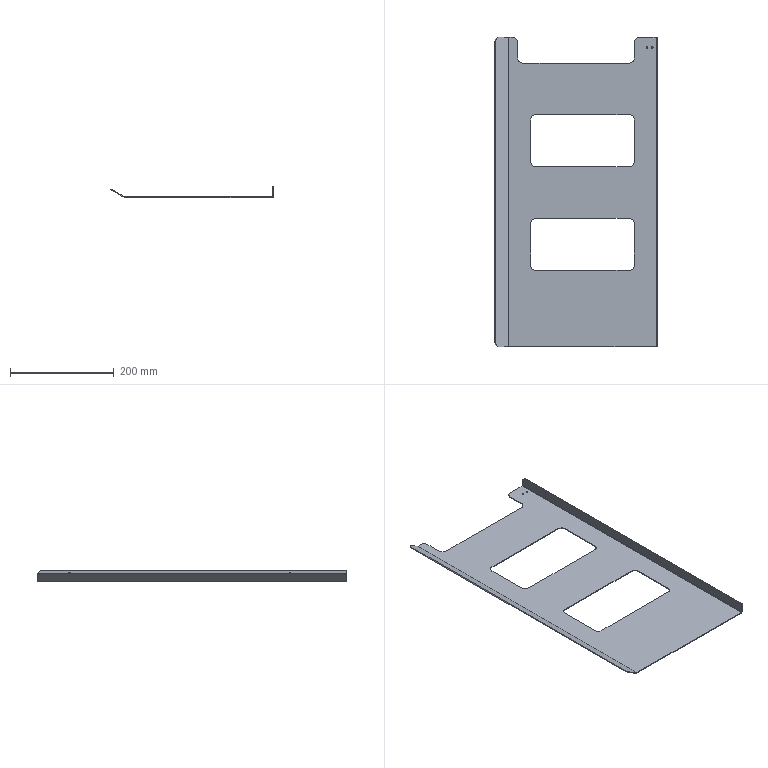Part | STEP file | PN_0004(Default) | 1 solid | 58 faces | box 313.731 x 597.76 x 21.5 mm | volume 225169 mm3 | plane 31 | cylinder 27 | commonest cylinder face diameters 20 x15 2.5 x4 4.2 x4 1.473 x2 4.473 x2